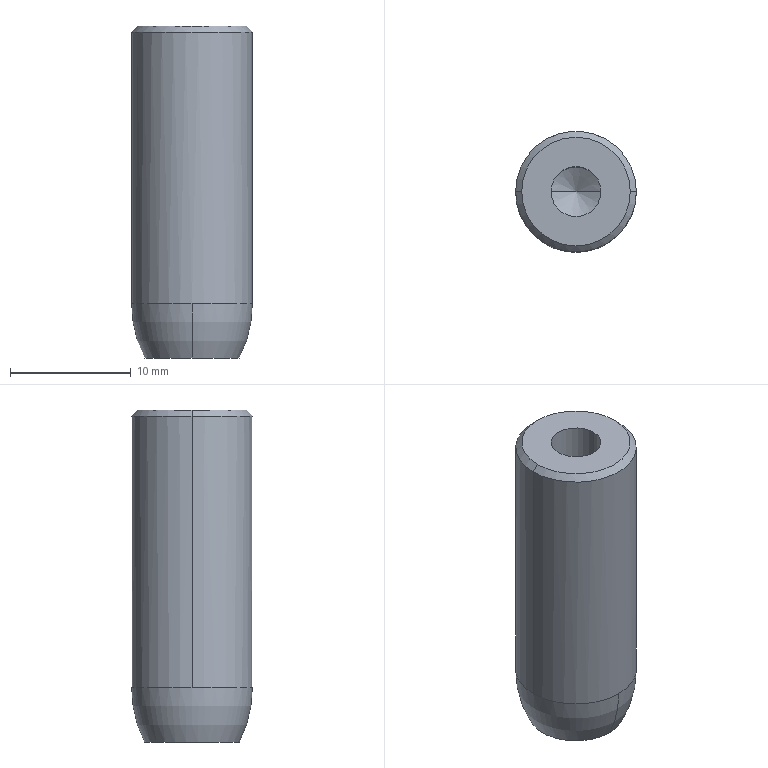Part | SolidWorks | features BaseBody 1 | 1 solid | 12 faces | box 10 x 10 x 27.5 mm | volume 1957 mm3 | cylinder 4 | cone 4 | torus 2 | plane 2 | commonest cylinder face diameters 4.134 x2 10 x2
STEP:
#1=CARTESIAN_POINT('',(0.,5.,-23.));
#2=VERTEX_POINT('',#1);
#3=CARTESIAN_POINT('',(-5.,0.,-23.));
#4=VERTEX_POINT('',#3);
#5=CARTESIAN_POINT('',(0.,0.,-23.));
#6=DIRECTION('',(0.,0.,1.));
#7=DIRECTION('',(1.,0.,0.));
#8=AXIS2_PLACEMENT_3D('',#5,#6,#7);
#9=CIRCLE('',#8,5.);
#10=EDGE_CURVE('',#2,#4,#9,.T.);
#11=ORIENTED_EDGE('',*,*,#10,.T.);
#12=CARTESIAN_POINT('',(-5.,0.,-0.5));
#13=VERTEX_POINT('',#12);
#14=CARTESIAN_POINT('',(-5.,0.,-27.5));
#15=DIRECTION('',(0.,0.,1.));
#16=VECTOR('',#15,1000.);
#17=LINE('',#14,#16);
#18=EDGE_CURVE('',#4,#13,#17,.T.);
#19=ORIENTED_EDGE('',*,*,#18,.T.);
#20=CARTESIAN_POINT('',(5.,0.,-0.5));
#21=VERTEX_POINT('',#20);
#22=CARTESIAN_POINT('',(0.,0.,-0.5));
#23=DIRECTION('',(0.,0.,-1.));
#24=DIRECTION('',(1.,0.,0.));
#25=AXIS2_PLACEMENT_3D('',#22,#23,#24);
#26=CIRCLE('',#25,5.);
#27=EDGE_CURVE('',#13,#21,#26,.T.);
#28=ORIENTED_EDGE('',*,*,#27,.T.);
#29=CARTESIAN_POINT('',(5.,0.,-23.));
#30=VERTEX_POINT('',#29);
#31=CARTESIAN_POINT('',(5.,0.,-27.5));
#32=DIRECTION('',(0.,0.,1.));
#33=VECTOR('',#32,1000.);
#34=LINE('',#31,#33);
#35=EDGE_CURVE('',#30,#21,#34,.T.);
#36=ORIENTED_EDGE('',*,*,#35,.F.);
#37=CARTESIAN_POINT('',(0.,0.,-23.));
#38=DIRECTION('',(0.,0.,1.));
#39=DIRECTION('',(1.,0.,0.));
#40=AXIS2_PLACEMENT_3D('',#37,#38,#39);
#41=CIRCLE('',#40,5.);
#42=EDGE_CURVE('',#30,#2,#41,.T.);
#43=ORIENTED_EDGE('',*,*,#42,.T.);
#44=EDGE_LOOP('',(#11,#19,#28,#36,#43));
#45=FACE_OUTER_BOUND('',#44,.T.);
#46=CARTESIAN_POINT('',(0.,0.,-27.5));
#47=DIRECTION('',(0.,0.,1.));
#48=DIRECTION('',(1.,0.,0.));
#49=AXIS2_PLACEMENT_3D('',#46,#47,#48);
#50=CYLINDRICAL_SURFACE('',#49,5.);
#51=ADVANCED_FACE('',(#45),#50,.T.);
#52=CARTESIAN_POINT('',(-4.5,0.,0.));
#53=VERTEX_POINT('',#52);
#54=CARTESIAN_POINT('',(4.5,0.,0.));
#55=VERTEX_POINT('',#54);
#56=CARTESIAN_POINT('',(0.,0.,0.));
#57=DIRECTION('',(0.,0.,-1.));
#58=DIRECTION('',(-1.,0.,0.));
#59=AXIS2_PLACEMENT_3D('',#56,#57,#58);
#60=CIRCLE('',#59,4.5);
#61=EDGE_CURVE('',#53,#55,#60,.T.);
#62=ORIENTED_EDGE('',*,*,#61,.T.);
#63=CARTESIAN_POINT('',(5.,0.,-0.5));
#64=DIRECTION('',(0.7071,0.,-0.7071));
#65=VECTOR('',#64,1000.);
#66=LINE('',#63,#65);
#67=EDGE_CURVE('',#55,#21,#66,.T.);
#68=ORIENTED_EDGE('',*,*,#67,.T.);
#69=ORIENTED_EDGE('',*,*,#27,.F.);
#70=CARTESIAN_POINT('',(-5.,0.,-0.5));
#71=DIRECTION('',(-0.7071,0.,-0.7071));
#72=VECTOR('',#71,1000.);
#73=LINE('',#70,#72);
#74=EDGE_CURVE('',#53,#13,#73,.T.);
#75=ORIENTED_EDGE('',*,*,#74,.F.);
#76=EDGE_LOOP('',(#62,#68,#69,#75));
#77=FACE_OUTER_BOUND('',#76,.T.);
#78=CARTESIAN_POINT('',(0.,0.,-0.5));
#79=DIRECTION('',(0.,0.,-1.));
#80=DIRECTION('',(-1.,0.,0.));
#81=AXIS2_PLACEMENT_3D('',#78,#79,#80);
#82=CONICAL_SURFACE('',#81,5.,0.7854);
#83=ADVANCED_FACE('',(#77),#82,.T.);
#84=CARTESIAN_POINT('',(0.,-5.,-23.));
#85=VERTEX_POINT('',#84);
#86=CARTESIAN_POINT('',(0.,0.,-23.));
#87=DIRECTION('',(0.,0.,1.));
#88=DIRECTION('',(1.,0.,0.));
#89=AXIS2_PLACEMENT_3D('',#86,#87,#88);
#90=CIRCLE('',#89,5.);
#91=EDGE_CURVE('',#85,#30,#90,.T.);
#92=ORIENTED_EDGE('',*,*,#91,.F.);
#93=CARTESIAN_POINT('',(0.,-3.93,-27.5));
#94=VERTEX_POINT('',#93);
#95=CARTESIAN_POINT('',(0.,5.,-23.));
#96=DIRECTION('',(1.,0.,0.));
#97=DIRECTION('',(0.,1.,0.));
#98=AXIS2_PLACEMENT_3D('',#95,#96,#97);
#99=CIRCLE('',#98,10.);
#100=EDGE_CURVE('',#85,#94,#99,.T.);
#101=ORIENTED_EDGE('',*,*,#100,.T.);
#102=CARTESIAN_POINT('',(0.,3.93,-27.5));
#103=VERTEX_POINT('',#102);
#104=CARTESIAN_POINT('',(0.,0.,-27.5));
#105=DIRECTION('',(0.,0.,1.));
#106=DIRECTION('',(0.,1.,0.));
#107=AXIS2_PLACEMENT_3D('',#104,#105,#106);
#108=CIRCLE('',#107,3.93);
#109=EDGE_CURVE('',#94,#103,#108,.T.);
#110=ORIENTED_EDGE('',*,*,#109,.T.);
#111=CARTESIAN_POINT('',(0.,-5.,-23.));
#112=DIRECTION('',(-1.,0.,0.));
#113=DIRECTION('',(0.,0.,1.));
#114=AXIS2_PLACEMENT_3D('',#111,#112,#113);
#115=CIRCLE('',#114,10.);
#116=EDGE_CURVE('',#2,#103,#115,.T.);
#117=ORIENTED_EDGE('',*,*,#116,.F.);
#118=ORIENTED_EDGE('',*,*,#42,.F.);
#119=EDGE_LOOP('',(#92,#101,#110,#117,#118));
#120=FACE_OUTER_BOUND('',#119,.T.);
#121=CARTESIAN_POINT('',(0.,0.,-23.));
#122=DIRECTION('',(0.,0.,-1.));
#123=DIRECTION('',(0.,1.,0.));
#124=AXIS2_PLACEMENT_3D('',#121,#122,#123);
#125=TOROIDAL_SURFACE('',#124,-5.,10.);
#126=ADVANCED_FACE('',(#120),#125,.T.);
#127=CARTESIAN_POINT('',(-2.067,0.,-11.));
#128=VERTEX_POINT('',#127);
#129=CARTESIAN_POINT('',(2.067,0.,-11.));
#130=VERTEX_POINT('',#129);
#131=CARTESIAN_POINT('',(0.,0.,-11.));
#132=DIRECTION('',(0.,0.,1.));
#133=DIRECTION('',(1.,0.,0.));
#134=AXIS2_PLACEMENT_3D('',#131,#132,#133);
#135=CIRCLE('',#134,2.067);
#136=EDGE_CURVE('',#128,#130,#135,.T.);
#137=ORIENTED_EDGE('',*,*,#136,.F.);
#138=CARTESIAN_POINT('',(-2.067,0.,0.));
#139=VERTEX_POINT('',#138);
#140=CARTESIAN_POINT('',(-2.067,0.,-27.5));
#141=DIRECTION('',(0.,0.,1.));
#142=VECTOR('',#141,1000.);
#143=LINE('',#140,#142);
#144=EDGE_CURVE('',#128,#139,#143,.T.);
#145=ORIENTED_EDGE('',*,*,#144,.T.);
#146=CARTESIAN_POINT('',(2.067,0.,0.));
#147=VERTEX_POINT('',#146);
#148=CARTESIAN_POINT('',(0.,0.,0.));
#149=DIRECTION('',(0.,0.,1.));
#150=DIRECTION('',(1.,0.,0.));
#151=AXIS2_PLACEMENT_3D('',#148,#149,#150);
#152=CIRCLE('',#151,2.067);
#153=EDGE_CURVE('',#139,#147,#152,.T.);
#154=ORIENTED_EDGE('',*,*,#153,.T.);
#155=CARTESIAN_POINT('',(2.067,0.,-27.5));
#156=DIRECTION('',(0.,0.,1.));
#157=VECTOR('',#156,1000.);
#158=LINE('',#155,#157);
#159=EDGE_CURVE('',#130,#147,#158,.T.);
#160=ORIENTED_EDGE('',*,*,#159,.F.);
#161=EDGE_LOOP('',(#137,#145,#154,#160));
#162=FACE_OUTER_BOUND('',#161,.T.);
#163=CARTESIAN_POINT('',(0.,0.,-27.5));
#164=DIRECTION('',(0.,0.,1.));
#165=DIRECTION('',(1.,0.,0.));
#166=AXIS2_PLACEMENT_3D('',#163,#164,#165);
#167=CYLINDRICAL_SURFACE('',#166,2.067);
#168=ADVANCED_FACE('',(#162),#167,.F.);
#169=CARTESIAN_POINT('',(0.,0.,-12.193));
#170=VERTEX_POINT('',#169);
#171=CARTESIAN_POINT('',(2.067,0.,-11.));
#172=DIRECTION('',(0.866,0.,0.5));
#173=VECTOR('',#172,1000.);
#174=LINE('',#171,#173);
#175=EDGE_CURVE('',#170,#130,#174,.T.);
#176=ORIENTED_EDGE('',*,*,#175,.F.);
#177=CARTESIAN_POINT('',(-2.067,0.,-11.));
#178=DIRECTION('',(-0.866,0.,0.5));
#179=VECTOR('',#178,1000.);
#180=LINE('',#177,#179);
#181=EDGE_CURVE('',#170,#128,#180,.T.);
#182=ORIENTED_EDGE('',*,*,#181,.T.);
#183=ORIENTED_EDGE('',*,*,#136,.T.);
#184=EDGE_LOOP('',(#176,#182,#183));
#185=FACE_OUTER_BOUND('',#184,.T.);
#186=CARTESIAN_POINT('',(0.,0.,-11.));
#187=DIRECTION('',(0.,0.,1.));
#188=DIRECTION('',(1.,0.,0.));
#189=AXIS2_PLACEMENT_3D('',#186,#187,#188);
#190=CONICAL_SURFACE('',#189,2.067,1.047);
#191=ADVANCED_FACE('',(#185),#190,.F.);
#192=ORIENTED_EDGE('',*,*,#18,.F.);
#193=CARTESIAN_POINT('',(0.,0.,-23.));
#194=DIRECTION('',(0.,0.,1.));
#195=DIRECTION('',(1.,0.,0.));
#196=AXIS2_PLACEMENT_3D('',#193,#194,#195);
#197=CIRCLE('',#196,5.);
#198=EDGE_CURVE('',#4,#85,#197,.T.);
#199=ORIENTED_EDGE('',*,*,#198,.T.);
#200=ORIENTED_EDGE('',*,*,#91,.T.);
#201=ORIENTED_EDGE('',*,*,#35,.T.);
#202=CARTESIAN_POINT('',(0.,0.,-0.5));
#203=DIRECTION('',(0.,0.,-1.));
#204=DIRECTION('',(1.,0.,0.));
#205=AXIS2_PLACEMENT_3D('',#202,#203,#204);
#206=CIRCLE('',#205,5.);
#207=EDGE_CURVE('',#21,#13,#206,.T.);
#208=ORIENTED_EDGE('',*,*,#207,.T.);
#209=EDGE_LOOP('',(#192,#199,#200,#201,#208));
#210=FACE_OUTER_BOUND('',#209,.T.);
#211=CARTESIAN_POINT('',(0.,0.,-27.5));
#212=DIRECTION('',(0.,0.,1.));
#213=DIRECTION('',(1.,0.,0.));
#214=AXIS2_PLACEMENT_3D('',#211,#212,#213);
#215=CYLINDRICAL_SURFACE('',#214,5.);
#216=ADVANCED_FACE('',(#210),#215,.T.);
#217=ORIENTED_EDGE('',*,*,#67,.F.);
#218=CARTESIAN_POINT('',(0.,0.,0.));
#219=DIRECTION('',(0.,0.,-1.));
#220=DIRECTION('',(-1.,0.,0.));
#221=AXIS2_PLACEMENT_3D('',#218,#219,#220);
#222=CIRCLE('',#221,4.5);
#223=EDGE_CURVE('',#55,#53,#222,.T.);
#224=ORIENTED_EDGE('',*,*,#223,.T.);
#225=ORIENTED_EDGE('',*,*,#74,.T.);
#226=ORIENTED_EDGE('',*,*,#207,.F.);
#227=EDGE_LOOP('',(#217,#224,#225,#226));
#228=FACE_OUTER_BOUND('',#227,.T.);
#229=CARTESIAN_POINT('',(0.,0.,-0.5));
#230=DIRECTION('',(0.,0.,-1.));
#231=DIRECTION('',(-1.,0.,0.));
#232=AXIS2_PLACEMENT_3D('',#229,#230,#231);
#233=CONICAL_SURFACE('',#232,5.,0.7854);
#234=ADVANCED_FACE('',(#228),#233,.T.);
#235=ORIENTED_EDGE('',*,*,#100,.F.);
#236=ORIENTED_EDGE('',*,*,#198,.F.);
#237=ORIENTED_EDGE('',*,*,#10,.F.);
#238=ORIENTED_EDGE('',*,*,#116,.T.);
#239=CARTESIAN_POINT('',(0.,0.,-27.5));
#240=DIRECTION('',(0.,0.,1.));
#241=DIRECTION('',(0.,1.,0.));
#242=AXIS2_PLACEMENT_3D('',#239,#240,#241);
#243=CIRCLE('',#242,3.93);
#244=EDGE_CURVE('',#103,#94,#243,.T.);
#245=ORIENTED_EDGE('',*,*,#244,.T.);
#246=EDGE_LOOP('',(#235,#236,#237,#238,#245));
#247=FACE_OUTER_BOUND('',#246,.T.);
#248=CARTESIAN_POINT('',(0.,0.,-23.));
#249=DIRECTION('',(0.,0.,-1.));
#250=DIRECTION('',(0.,1.,0.));
#251=AXIS2_PLACEMENT_3D('',#248,#249,#250);
#252=TOROIDAL_SURFACE('',#251,-5.,10.);
#253=ADVANCED_FACE('',(#247),#252,.T.);
#254=CARTESIAN_POINT('',(0.,0.,0.));
#255=DIRECTION('',(0.,0.,1.));
#256=DIRECTION('',(1.,0.,0.));
#257=AXIS2_PLACEMENT_3D('',#254,#255,#256);
#258=CIRCLE('',#257,2.067);
#259=EDGE_CURVE('',#147,#139,#258,.T.);
#260=ORIENTED_EDGE('',*,*,#259,.F.);
#261=ORIENTED_EDGE('',*,*,#153,.F.);
#262=EDGE_LOOP('',(#260,#261));
#263=FACE_BOUND('',#262,.T.);
#264=ORIENTED_EDGE('',*,*,#61,.F.);
#265=ORIENTED_EDGE('',*,*,#223,.F.);
#266=EDGE_LOOP('',(#264,#265));
#267=FACE_OUTER_BOUND('',#266,.T.);
#268=CARTESIAN_POINT('',(0.,2.067,0.));
#269=DIRECTION('',(0.,0.,-1.));
#270=DIRECTION('',(-1.,0.,0.));
#271=AXIS2_PLACEMENT_3D('',#268,#269,#270);
#272=PLANE('',#271);
#273=ADVANCED_FACE('',(#263,#267),#272,.F.);
#274=ORIENTED_EDGE('',*,*,#244,.F.);
#275=ORIENTED_EDGE('',*,*,#109,.F.);
#276=EDGE_LOOP('',(#274,#275));
#277=FACE_OUTER_BOUND('',#276,.T.);
#278=CARTESIAN_POINT('',(0.,3.93,-27.5));
#279=DIRECTION('',(0.,0.,1.));
#280=DIRECTION('',(1.,0.,0.));
#281=AXIS2_PLACEMENT_3D('',#278,#279,#280);
#282=PLANE('',#281);
#283=ADVANCED_FACE('',(#277),#282,.F.);
#284=ORIENTED_EDGE('',*,*,#144,.F.);
#285=CARTESIAN_POINT('',(0.,0.,-11.));
#286=DIRECTION('',(0.,0.,1.));
#287=DIRECTION('',(1.,0.,0.));
#288=AXIS2_PLACEMENT_3D('',#285,#286,#287);
#289=CIRCLE('',#288,2.067);
#290=EDGE_CURVE('',#130,#128,#289,.T.);
#291=ORIENTED_EDGE('',*,*,#290,.F.);
#292=ORIENTED_EDGE('',*,*,#159,.T.);
#293=ORIENTED_EDGE('',*,*,#259,.T.);
#294=EDGE_LOOP('',(#284,#291,#292,#293));
#295=FACE_OUTER_BOUND('',#294,.T.);
#296=CARTESIAN_POINT('',(0.,0.,-27.5));
#297=DIRECTION('',(0.,0.,1.));
#298=DIRECTION('',(1.,0.,0.));
#299=AXIS2_PLACEMENT_3D('',#296,#297,#298);
#300=CYLINDRICAL_SURFACE('',#299,2.067);
#301=ADVANCED_FACE('',(#295),#300,.F.);
#302=ORIENTED_EDGE('',*,*,#181,.F.);
#303=ORIENTED_EDGE('',*,*,#175,.T.);
#304=ORIENTED_EDGE('',*,*,#290,.T.);
#305=EDGE_LOOP('',(#302,#303,#304));
#306=FACE_OUTER_BOUND('',#305,.T.);
#307=CARTESIAN_POINT('',(0.,0.,-11.));
#308=DIRECTION('',(0.,0.,1.));
#309=DIRECTION('',(1.,0.,0.));
#310=AXIS2_PLACEMENT_3D('',#307,#308,#309);
#311=CONICAL_SURFACE('',#310,2.067,1.047);
#312=ADVANCED_FACE('',(#306),#311,.F.);
#313=CLOSED_SHELL('',(#51,#83,#126,#168,#191,#216,#234,#253,#273,#283,#301,#312));
#314=MANIFOLD_SOLID_BREP('',#313);
#315=CARTESIAN_POINT('',(0.,0.,0.));
#316=DIRECTION('',(0.,0.,1.));
#317=DIRECTION('',(1.,0.,0.));
#318=AXIS2_PLACEMENT_3D('',#315,#316,#317);
#319=(LENGTH_UNIT()NAMED_UNIT(*)SI_UNIT(.MILLI.,.METRE.));
#320=UNCERTAINTY_MEASURE_WITH_UNIT(LENGTH_MEASURE(0.00001),#319,'','');
#321=(NAMED_UNIT(*)PLANE_ANGLE_UNIT()SI_UNIT($,.RADIAN.));
#322=(NAMED_UNIT(*)SI_UNIT($,.STERADIAN.)SOLID_ANGLE_UNIT());
#323=(GEOMETRIC_REPRESENTATION_CONTEXT(3)GLOBAL_UNCERTAINTY_ASSIGNED_CONTEXT((#320))GLOBAL_UNIT_ASSIGNED_CONTEXT((#319,#321,#322))REPRESENTATION_CONTEXT('',''));
#324=ADVANCED_BREP_SHAPE_REPRESENTATION('',(#314,#318),#323);